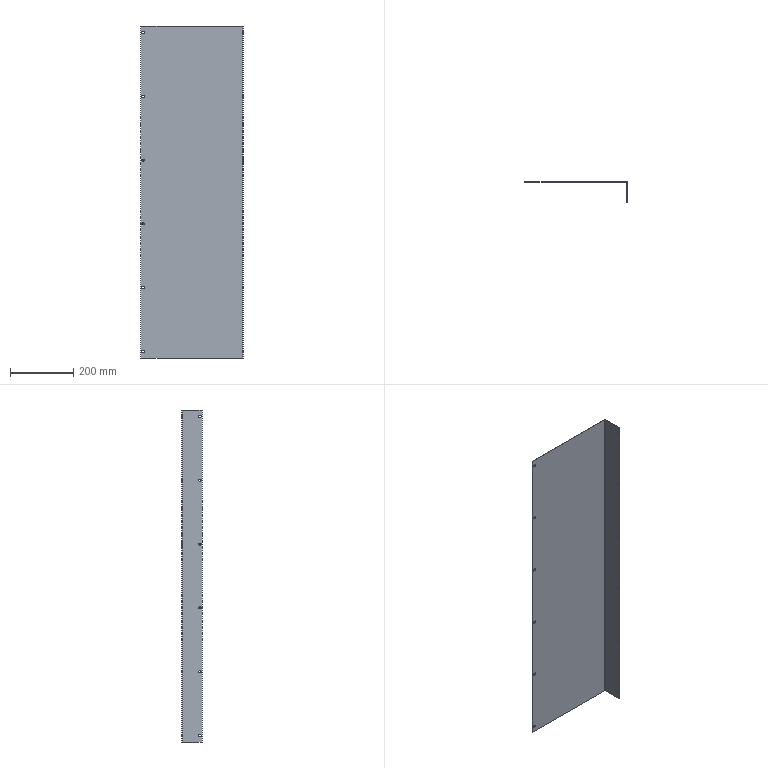Part | SolidWorks | features ICE 2, FlatPattern 1, SMBaseFlange 1, SheetMetal 1 | 1 solid | 74 faces | box 323.5 x 64 x 1050 mm | volume 404954 mm3 | cylinder 38 | plane 36 | commonest cylinder face diameters 6 x36 0.4 x1 2.4 x1